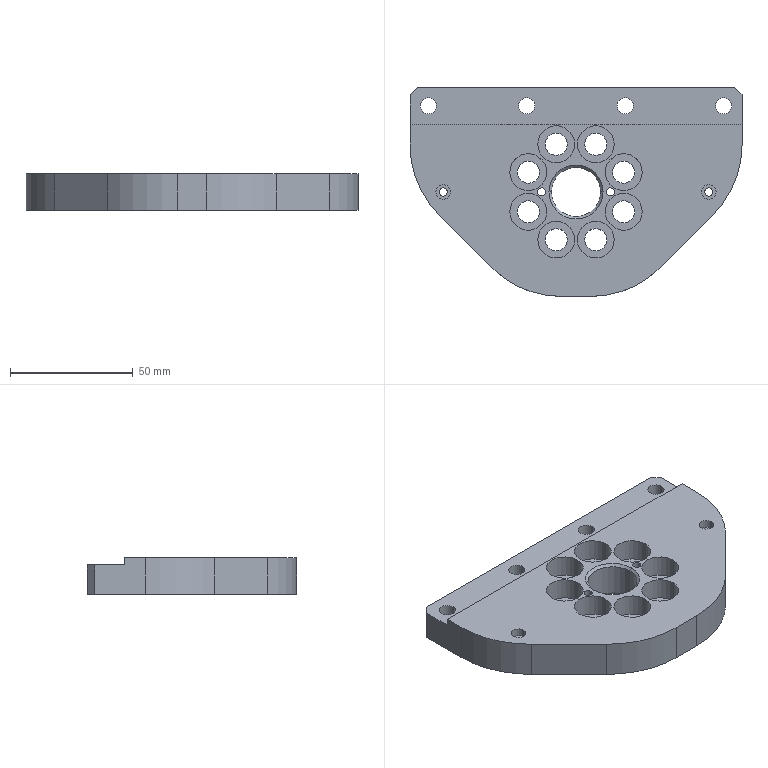Part | SolidWorks | features HoleWzd 5, Chamfer 2, CirPattern 1, Extrusion 1, ICE 1 | 1 solid | 104 faces | box 135 x 85 x 15 mm | volume 108283 mm3 | cylinder 70 | plane 26 | cone 8 | commonest cylinder face diameters 9 x16 15 x16 6.6 x8 11 x8 3.3 x4 3.4 x4